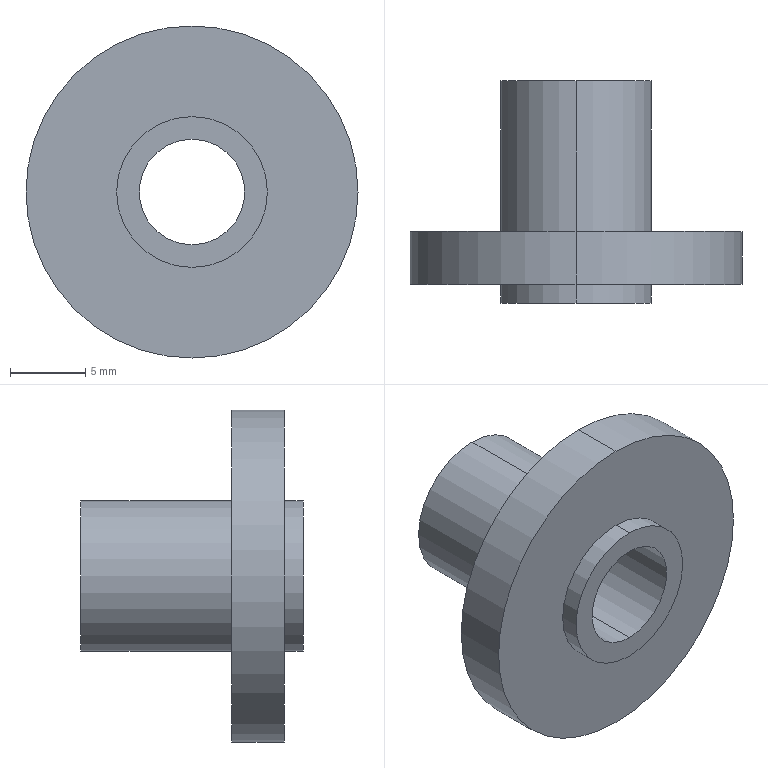Part | SolidWorks | features ICE 2, 3DProfileFeature 1, Extrusion 1, HoleWzd 1 | 1 solid | 12 faces | box 22 x 14.75 x 22 mm | volume 1646 mm3 | cylinder 8 | plane 4 | commonest cylinder face diameters 10 x4 7 x2 22 x2
STEP:
#1=CARTESIAN_POINT('',(0.,-1.25,-3.5));
#2=VERTEX_POINT('',#1);
#3=CARTESIAN_POINT('',(0.,-1.25,3.5));
#4=VERTEX_POINT('',#3);
#5=CARTESIAN_POINT('',(0.,-1.25,0.));
#6=DIRECTION('',(0.,1.,0.));
#7=DIRECTION('',(0.,0.,1.));
#8=AXIS2_PLACEMENT_3D('',#5,#6,#7);
#9=CIRCLE('',#8,3.5);
#10=EDGE_CURVE('',#2,#4,#9,.T.);
#11=ORIENTED_EDGE('',*,*,#10,.F.);
#12=CARTESIAN_POINT('',(0.,13.5,-3.5));
#13=VERTEX_POINT('',#12);
#14=CARTESIAN_POINT('',(0.,13.5,-3.5));
#15=DIRECTION('',(0.,1.,0.));
#16=VECTOR('',#15,1000.);
#17=LINE('',#14,#16);
#18=EDGE_CURVE('',#2,#13,#17,.T.);
#19=ORIENTED_EDGE('',*,*,#18,.T.);
#20=CARTESIAN_POINT('',(0.,13.5,3.5));
#21=VERTEX_POINT('',#20);
#22=CARTESIAN_POINT('',(0.,13.5,0.));
#23=DIRECTION('',(0.,1.,0.));
#24=DIRECTION('',(0.,0.,1.));
#25=AXIS2_PLACEMENT_3D('',#22,#23,#24);
#26=CIRCLE('',#25,3.5);
#27=EDGE_CURVE('',#13,#21,#26,.T.);
#28=ORIENTED_EDGE('',*,*,#27,.T.);
#29=CARTESIAN_POINT('',(0.,13.5,3.5));
#30=DIRECTION('',(0.,1.,0.));
#31=VECTOR('',#30,1000.);
#32=LINE('',#29,#31);
#33=EDGE_CURVE('',#4,#21,#32,.T.);
#34=ORIENTED_EDGE('',*,*,#33,.F.);
#35=EDGE_LOOP('',(#11,#19,#28,#34));
#36=FACE_OUTER_BOUND('',#35,.T.);
#37=CARTESIAN_POINT('',(0.,13.5,0.));
#38=DIRECTION('',(0.,1.,0.));
#39=DIRECTION('',(0.,0.,1.));
#40=AXIS2_PLACEMENT_3D('',#37,#38,#39);
#41=CYLINDRICAL_SURFACE('',#40,3.5);
#42=ADVANCED_FACE('',(#36),#41,.F.);
#43=CARTESIAN_POINT('',(0.,-1.25,5.));
#44=VERTEX_POINT('',#43);
#45=CARTESIAN_POINT('',(0.,-1.25,-5.));
#46=VERTEX_POINT('',#45);
#47=CARTESIAN_POINT('',(0.,-1.25,0.));
#48=DIRECTION('',(0.,1.,0.));
#49=DIRECTION('',(0.,0.,1.));
#50=AXIS2_PLACEMENT_3D('',#47,#48,#49);
#51=CIRCLE('',#50,5.);
#52=EDGE_CURVE('',#44,#46,#51,.T.);
#53=ORIENTED_EDGE('',*,*,#52,.T.);
#54=CARTESIAN_POINT('',(0.,0.,-5.));
#55=VERTEX_POINT('',#54);
#56=CARTESIAN_POINT('',(0.,-1.25,-5.));
#57=DIRECTION('',(0.,1.,0.));
#58=VECTOR('',#57,1000.);
#59=LINE('',#56,#58);
#60=EDGE_CURVE('',#46,#55,#59,.T.);
#61=ORIENTED_EDGE('',*,*,#60,.T.);
#62=CARTESIAN_POINT('',(0.,0.,5.));
#63=VERTEX_POINT('',#62);
#64=CARTESIAN_POINT('',(0.,0.,0.));
#65=DIRECTION('',(0.,1.,0.));
#66=DIRECTION('',(0.,0.,1.));
#67=AXIS2_PLACEMENT_3D('',#64,#65,#66);
#68=CIRCLE('',#67,5.);
#69=EDGE_CURVE('',#63,#55,#68,.T.);
#70=ORIENTED_EDGE('',*,*,#69,.F.);
#71=CARTESIAN_POINT('',(0.,-1.25,5.));
#72=DIRECTION('',(0.,1.,0.));
#73=VECTOR('',#72,1000.);
#74=LINE('',#71,#73);
#75=EDGE_CURVE('',#44,#63,#74,.T.);
#76=ORIENTED_EDGE('',*,*,#75,.F.);
#77=EDGE_LOOP('',(#53,#61,#70,#76));
#78=FACE_OUTER_BOUND('',#77,.T.);
#79=CARTESIAN_POINT('',(0.,-1.25,0.));
#80=DIRECTION('',(0.,1.,0.));
#81=DIRECTION('',(0.,0.,1.));
#82=AXIS2_PLACEMENT_3D('',#79,#80,#81);
#83=CYLINDRICAL_SURFACE('',#82,5.);
#84=ADVANCED_FACE('',(#78),#83,.T.);
#85=CARTESIAN_POINT('',(0.,13.5,5.));
#86=VERTEX_POINT('',#85);
#87=CARTESIAN_POINT('',(0.,13.5,-5.));
#88=VERTEX_POINT('',#87);
#89=CARTESIAN_POINT('',(0.,13.5,0.));
#90=DIRECTION('',(0.,1.,0.));
#91=DIRECTION('',(0.,0.,1.));
#92=AXIS2_PLACEMENT_3D('',#89,#90,#91);
#93=CIRCLE('',#92,5.);
#94=EDGE_CURVE('',#86,#88,#93,.T.);
#95=ORIENTED_EDGE('',*,*,#94,.F.);
#96=CARTESIAN_POINT('',(0.,3.5,5.));
#97=VERTEX_POINT('',#96);
#98=CARTESIAN_POINT('',(0.,13.5,5.));
#99=DIRECTION('',(0.,-1.,0.));
#100=VECTOR('',#99,1000.);
#101=LINE('',#98,#100);
#102=EDGE_CURVE('',#86,#97,#101,.T.);
#103=ORIENTED_EDGE('',*,*,#102,.T.);
#104=CARTESIAN_POINT('',(0.,3.5,-5.));
#105=VERTEX_POINT('',#104);
#106=CARTESIAN_POINT('',(0.,3.5,0.));
#107=DIRECTION('',(0.,1.,0.));
#108=DIRECTION('',(0.,0.,1.));
#109=AXIS2_PLACEMENT_3D('',#106,#107,#108);
#110=CIRCLE('',#109,5.);
#111=EDGE_CURVE('',#97,#105,#110,.T.);
#112=ORIENTED_EDGE('',*,*,#111,.T.);
#113=CARTESIAN_POINT('',(0.,13.5,-5.));
#114=DIRECTION('',(0.,-1.,0.));
#115=VECTOR('',#114,1000.);
#116=LINE('',#113,#115);
#117=EDGE_CURVE('',#88,#105,#116,.T.);
#118=ORIENTED_EDGE('',*,*,#117,.F.);
#119=EDGE_LOOP('',(#95,#103,#112,#118));
#120=FACE_OUTER_BOUND('',#119,.T.);
#121=CARTESIAN_POINT('',(0.,13.5,0.));
#122=DIRECTION('',(0.,-1.,0.));
#123=DIRECTION('',(0.,0.,-1.));
#124=AXIS2_PLACEMENT_3D('',#121,#122,#123);
#125=CYLINDRICAL_SURFACE('',#124,5.);
#126=ADVANCED_FACE('',(#120),#125,.T.);
#127=CARTESIAN_POINT('',(0.,3.5,11.));
#128=VERTEX_POINT('',#127);
#129=CARTESIAN_POINT('',(0.,3.5,-11.));
#130=VERTEX_POINT('',#129);
#131=CARTESIAN_POINT('',(0.,3.5,0.));
#132=DIRECTION('',(0.,1.,0.));
#133=DIRECTION('',(0.,0.,1.));
#134=AXIS2_PLACEMENT_3D('',#131,#132,#133);
#135=CIRCLE('',#134,11.);
#136=EDGE_CURVE('',#128,#130,#135,.T.);
#137=ORIENTED_EDGE('',*,*,#136,.F.);
#138=CARTESIAN_POINT('',(0.,0.,11.));
#139=VERTEX_POINT('',#138);
#140=CARTESIAN_POINT('',(0.,3.5,11.));
#141=DIRECTION('',(0.,-1.,0.));
#142=VECTOR('',#141,1000.);
#143=LINE('',#140,#142);
#144=EDGE_CURVE('',#128,#139,#143,.T.);
#145=ORIENTED_EDGE('',*,*,#144,.T.);
#146=CARTESIAN_POINT('',(0.,0.,-11.));
#147=VERTEX_POINT('',#146);
#148=CARTESIAN_POINT('',(0.,0.,0.));
#149=DIRECTION('',(0.,1.,0.));
#150=DIRECTION('',(0.,0.,1.));
#151=AXIS2_PLACEMENT_3D('',#148,#149,#150);
#152=CIRCLE('',#151,11.);
#153=EDGE_CURVE('',#139,#147,#152,.T.);
#154=ORIENTED_EDGE('',*,*,#153,.T.);
#155=CARTESIAN_POINT('',(0.,3.5,-11.));
#156=DIRECTION('',(0.,-1.,0.));
#157=VECTOR('',#156,1000.);
#158=LINE('',#155,#157);
#159=EDGE_CURVE('',#130,#147,#158,.T.);
#160=ORIENTED_EDGE('',*,*,#159,.F.);
#161=EDGE_LOOP('',(#137,#145,#154,#160));
#162=FACE_OUTER_BOUND('',#161,.T.);
#163=CARTESIAN_POINT('',(0.,3.5,0.));
#164=DIRECTION('',(0.,-1.,0.));
#165=DIRECTION('',(0.,0.,-1.));
#166=AXIS2_PLACEMENT_3D('',#163,#164,#165);
#167=CYLINDRICAL_SURFACE('',#166,11.);
#168=ADVANCED_FACE('',(#162),#167,.T.);
#169=CARTESIAN_POINT('',(0.,3.5,0.));
#170=DIRECTION('',(0.,1.,0.));
#171=DIRECTION('',(0.,0.,1.));
#172=AXIS2_PLACEMENT_3D('',#169,#170,#171);
#173=CIRCLE('',#172,11.);
#174=EDGE_CURVE('',#130,#128,#173,.T.);
#175=ORIENTED_EDGE('',*,*,#174,.T.);
#176=ORIENTED_EDGE('',*,*,#136,.T.);
#177=EDGE_LOOP('',(#175,#176));
#178=FACE_OUTER_BOUND('',#177,.T.);
#179=CARTESIAN_POINT('',(0.,3.5,0.));
#180=DIRECTION('',(0.,1.,0.));
#181=DIRECTION('',(0.,0.,1.));
#182=AXIS2_PLACEMENT_3D('',#179,#180,#181);
#183=CIRCLE('',#182,5.);
#184=EDGE_CURVE('',#105,#97,#183,.T.);
#185=ORIENTED_EDGE('',*,*,#184,.F.);
#186=ORIENTED_EDGE('',*,*,#111,.F.);
#187=EDGE_LOOP('',(#185,#186));
#188=FACE_BOUND('',#187,.T.);
#189=CARTESIAN_POINT('',(0.,3.5,0.));
#190=DIRECTION('',(0.,1.,0.));
#191=DIRECTION('',(0.,0.,1.));
#192=AXIS2_PLACEMENT_3D('',#189,#190,#191);
#193=PLANE('',#192);
#194=ADVANCED_FACE('',(#178,#188),#193,.T.);
#195=ORIENTED_EDGE('',*,*,#69,.T.);
#196=CARTESIAN_POINT('',(0.,0.,0.));
#197=DIRECTION('',(0.,1.,0.));
#198=DIRECTION('',(0.,0.,1.));
#199=AXIS2_PLACEMENT_3D('',#196,#197,#198);
#200=CIRCLE('',#199,5.);
#201=EDGE_CURVE('',#55,#63,#200,.T.);
#202=ORIENTED_EDGE('',*,*,#201,.T.);
#203=EDGE_LOOP('',(#195,#202));
#204=FACE_BOUND('',#203,.T.);
#205=CARTESIAN_POINT('',(0.,0.,0.));
#206=DIRECTION('',(0.,1.,0.));
#207=DIRECTION('',(0.,0.,1.));
#208=AXIS2_PLACEMENT_3D('',#205,#206,#207);
#209=CIRCLE('',#208,11.);
#210=EDGE_CURVE('',#147,#139,#209,.T.);
#211=ORIENTED_EDGE('',*,*,#210,.F.);
#212=ORIENTED_EDGE('',*,*,#153,.F.);
#213=EDGE_LOOP('',(#211,#212));
#214=FACE_OUTER_BOUND('',#213,.T.);
#215=CARTESIAN_POINT('',(0.,0.,0.));
#216=DIRECTION('',(0.,1.,0.));
#217=DIRECTION('',(0.,0.,1.));
#218=AXIS2_PLACEMENT_3D('',#215,#216,#217);
#219=PLANE('',#218);
#220=ADVANCED_FACE('',(#204,#214),#219,.F.);
#221=ORIENTED_EDGE('',*,*,#144,.F.);
#222=ORIENTED_EDGE('',*,*,#174,.F.);
#223=ORIENTED_EDGE('',*,*,#159,.T.);
#224=ORIENTED_EDGE('',*,*,#210,.T.);
#225=EDGE_LOOP('',(#221,#222,#223,#224));
#226=FACE_OUTER_BOUND('',#225,.T.);
#227=CARTESIAN_POINT('',(0.,3.5,0.));
#228=DIRECTION('',(0.,-1.,0.));
#229=DIRECTION('',(0.,0.,-1.));
#230=AXIS2_PLACEMENT_3D('',#227,#228,#229);
#231=CYLINDRICAL_SURFACE('',#230,11.);
#232=ADVANCED_FACE('',(#226),#231,.T.);
#233=ORIENTED_EDGE('',*,*,#102,.F.);
#234=CARTESIAN_POINT('',(0.,13.5,0.));
#235=DIRECTION('',(0.,1.,0.));
#236=DIRECTION('',(0.,0.,1.));
#237=AXIS2_PLACEMENT_3D('',#234,#235,#236);
#238=CIRCLE('',#237,5.);
#239=EDGE_CURVE('',#88,#86,#238,.T.);
#240=ORIENTED_EDGE('',*,*,#239,.F.);
#241=ORIENTED_EDGE('',*,*,#117,.T.);
#242=ORIENTED_EDGE('',*,*,#184,.T.);
#243=EDGE_LOOP('',(#233,#240,#241,#242));
#244=FACE_OUTER_BOUND('',#243,.T.);
#245=CARTESIAN_POINT('',(0.,13.5,0.));
#246=DIRECTION('',(0.,-1.,0.));
#247=DIRECTION('',(0.,0.,-1.));
#248=AXIS2_PLACEMENT_3D('',#245,#246,#247);
#249=CYLINDRICAL_SURFACE('',#248,5.);
#250=ADVANCED_FACE('',(#244),#249,.T.);
#251=CARTESIAN_POINT('',(0.,13.5,0.));
#252=DIRECTION('',(0.,1.,0.));
#253=DIRECTION('',(0.,0.,1.));
#254=AXIS2_PLACEMENT_3D('',#251,#252,#253);
#255=CIRCLE('',#254,3.5);
#256=EDGE_CURVE('',#21,#13,#255,.T.);
#257=ORIENTED_EDGE('',*,*,#256,.F.);
#258=ORIENTED_EDGE('',*,*,#27,.F.);
#259=EDGE_LOOP('',(#257,#258));
#260=FACE_BOUND('',#259,.T.);
#261=ORIENTED_EDGE('',*,*,#239,.T.);
#262=ORIENTED_EDGE('',*,*,#94,.T.);
#263=EDGE_LOOP('',(#261,#262));
#264=FACE_OUTER_BOUND('',#263,.T.);
#265=CARTESIAN_POINT('',(0.,13.5,0.));
#266=DIRECTION('',(0.,1.,0.));
#267=DIRECTION('',(0.,0.,1.));
#268=AXIS2_PLACEMENT_3D('',#265,#266,#267);
#269=PLANE('',#268);
#270=ADVANCED_FACE('',(#260,#264),#269,.T.);
#271=ORIENTED_EDGE('',*,*,#60,.F.);
#272=CARTESIAN_POINT('',(0.,-1.25,0.));
#273=DIRECTION('',(0.,1.,0.));
#274=DIRECTION('',(0.,0.,1.));
#275=AXIS2_PLACEMENT_3D('',#272,#273,#274);
#276=CIRCLE('',#275,5.);
#277=EDGE_CURVE('',#46,#44,#276,.T.);
#278=ORIENTED_EDGE('',*,*,#277,.T.);
#279=ORIENTED_EDGE('',*,*,#75,.T.);
#280=ORIENTED_EDGE('',*,*,#201,.F.);
#281=EDGE_LOOP('',(#271,#278,#279,#280));
#282=FACE_OUTER_BOUND('',#281,.T.);
#283=CARTESIAN_POINT('',(0.,-1.25,0.));
#284=DIRECTION('',(0.,1.,0.));
#285=DIRECTION('',(0.,0.,1.));
#286=AXIS2_PLACEMENT_3D('',#283,#284,#285);
#287=CYLINDRICAL_SURFACE('',#286,5.);
#288=ADVANCED_FACE('',(#282),#287,.T.);
#289=CARTESIAN_POINT('',(0.,-1.25,0.));
#290=DIRECTION('',(0.,1.,0.));
#291=DIRECTION('',(0.,0.,1.));
#292=AXIS2_PLACEMENT_3D('',#289,#290,#291);
#293=CIRCLE('',#292,3.5);
#294=EDGE_CURVE('',#4,#2,#293,.T.);
#295=ORIENTED_EDGE('',*,*,#294,.T.);
#296=ORIENTED_EDGE('',*,*,#10,.T.);
#297=EDGE_LOOP('',(#295,#296));
#298=FACE_BOUND('',#297,.T.);
#299=ORIENTED_EDGE('',*,*,#52,.F.);
#300=ORIENTED_EDGE('',*,*,#277,.F.);
#301=EDGE_LOOP('',(#299,#300));
#302=FACE_OUTER_BOUND('',#301,.T.);
#303=CARTESIAN_POINT('',(0.,-1.25,0.));
#304=DIRECTION('',(0.,1.,0.));
#305=DIRECTION('',(0.,0.,1.));
#306=AXIS2_PLACEMENT_3D('',#303,#304,#305);
#307=PLANE('',#306);
#308=ADVANCED_FACE('',(#298,#302),#307,.F.);
#309=ORIENTED_EDGE('',*,*,#18,.F.);
#310=ORIENTED_EDGE('',*,*,#294,.F.);
#311=ORIENTED_EDGE('',*,*,#33,.T.);
#312=ORIENTED_EDGE('',*,*,#256,.T.);
#313=EDGE_LOOP('',(#309,#310,#311,#312));
#314=FACE_OUTER_BOUND('',#313,.T.);
#315=CARTESIAN_POINT('',(0.,13.5,0.));
#316=DIRECTION('',(0.,1.,0.));
#317=DIRECTION('',(0.,0.,1.));
#318=AXIS2_PLACEMENT_3D('',#315,#316,#317);
#319=CYLINDRICAL_SURFACE('',#318,3.5);
#320=ADVANCED_FACE('',(#314),#319,.F.);
#321=CLOSED_SHELL('',(#42,#84,#126,#168,#194,#220,#232,#250,#270,#288,#308,#320));
#322=MANIFOLD_SOLID_BREP('',#321);
#323=CARTESIAN_POINT('',(0.,0.,0.));
#324=DIRECTION('',(0.,0.,1.));
#325=DIRECTION('',(1.,0.,0.));
#326=AXIS2_PLACEMENT_3D('',#323,#324,#325);
#327=(LENGTH_UNIT()NAMED_UNIT(*)SI_UNIT(.MILLI.,.METRE.));
#328=UNCERTAINTY_MEASURE_WITH_UNIT(LENGTH_MEASURE(0.00001),#327,'','');
#329=(NAMED_UNIT(*)PLANE_ANGLE_UNIT()SI_UNIT($,.RADIAN.));
#330=(NAMED_UNIT(*)SI_UNIT($,.STERADIAN.)SOLID_ANGLE_UNIT());
#331=(GEOMETRIC_REPRESENTATION_CONTEXT(3)GLOBAL_UNCERTAINTY_ASSIGNED_CONTEXT((#328))GLOBAL_UNIT_ASSIGNED_CONTEXT((#327,#329,#330))REPRESENTATION_CONTEXT('',''));
#332=ADVANCED_BREP_SHAPE_REPRESENTATION('',(#322,#326),#331);